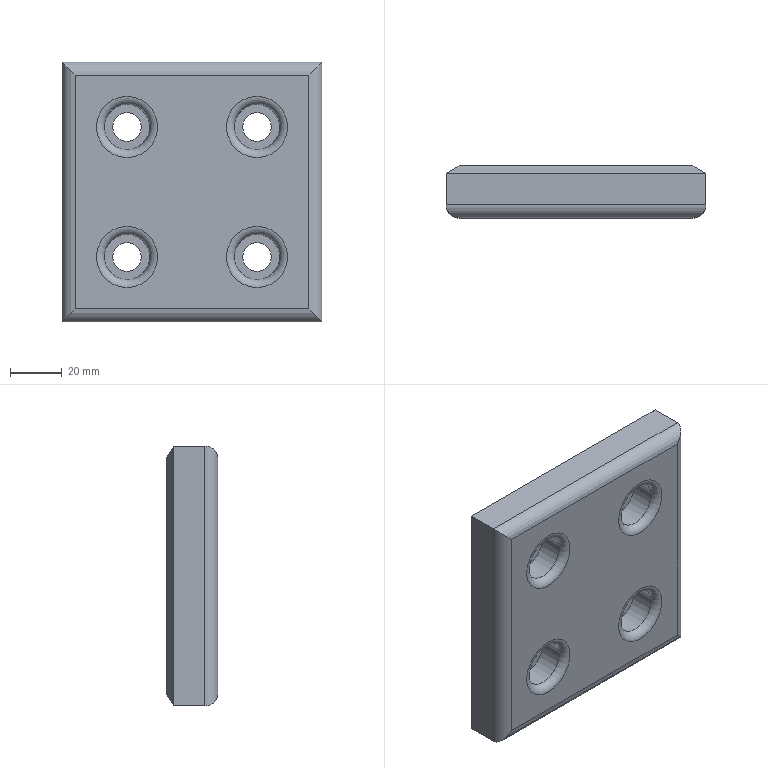Part | NX | features solid 2 | 1 solid | 30 faces | box 100 x 20 x 100 mm | volume 179958 mm3 | plane 14 | cylinder 12 | torus 4 | commonest cylinder face diameters 10 x4 11 x4 17.5 x4
STEP:
#1=CARTESIAN_POINT('',(395.,-583.,40.));
#2=VERTEX_POINT('',#1);
#3=CARTESIAN_POINT('',(395.,-595.,40.));
#4=VERTEX_POINT('',#3);
#5=CARTESIAN_POINT('',(395.,-580.,40.));
#6=DIRECTION('',(0.,-1.,0.));
#7=VECTOR('',#6,1000.);
#8=LINE('',#5,#7);
#9=EDGE_CURVE('',#2,#4,#8,.T.);
#10=ORIENTED_EDGE('',*,*,#9,.T.);
#11=CARTESIAN_POINT('',(395.,-595.,-60.));
#12=VERTEX_POINT('',#11);
#13=CARTESIAN_POINT('',(395.,-595.,90.));
#14=DIRECTION('',(0.,0.,-1.));
#15=VECTOR('',#14,1000.);
#16=LINE('',#13,#15);
#17=EDGE_CURVE('',#12,#4,#16,.F.);
#18=ORIENTED_EDGE('',*,*,#17,.F.);
#19=CARTESIAN_POINT('',(395.,-583.,-60.));
#20=VERTEX_POINT('',#19);
#21=CARTESIAN_POINT('',(395.,-580.,-60.));
#22=DIRECTION('',(0.,-1.,0.));
#23=VECTOR('',#22,1000.);
#24=LINE('',#21,#23);
#25=EDGE_CURVE('',#20,#12,#24,.T.);
#26=ORIENTED_EDGE('',*,*,#25,.F.);
#27=CARTESIAN_POINT('',(395.,-583.,-60.));
#28=DIRECTION('',(0.,0.,-1.));
#29=VECTOR('',#28,1000.);
#30=LINE('',#27,#29);
#31=EDGE_CURVE('',#2,#20,#30,.T.);
#32=ORIENTED_EDGE('',*,*,#31,.F.);
#33=EDGE_LOOP('',(#10,#18,#26,#32));
#34=FACE_BOUND('',#33,.T.);
#35=CARTESIAN_POINT('',(395.,-580.,90.));
#36=DIRECTION('',(1.,0.,0.));
#37=DIRECTION('',(0.,0.,1.));
#38=AXIS2_PLACEMENT_3D('',#35,#36,#37);
#39=PLANE('',#38);
#40=ADVANCED_FACE('',(#34),#39,.T.);
#41=CARTESIAN_POINT('',(295.,-583.,40.));
#42=VERTEX_POINT('',#41);
#43=CARTESIAN_POINT('',(295.,-595.,40.));
#44=VERTEX_POINT('',#43);
#45=CARTESIAN_POINT('',(295.,-580.,40.));
#46=DIRECTION('',(0.,-1.,0.));
#47=VECTOR('',#46,1000.);
#48=LINE('',#45,#47);
#49=EDGE_CURVE('',#42,#44,#48,.T.);
#50=ORIENTED_EDGE('',*,*,#49,.T.);
#51=CARTESIAN_POINT('',(295.,-595.,40.));
#52=DIRECTION('',(-1.,0.,0.));
#53=VECTOR('',#52,1000.);
#54=LINE('',#51,#53);
#55=EDGE_CURVE('',#4,#44,#54,.T.);
#56=ORIENTED_EDGE('',*,*,#55,.F.);
#57=ORIENTED_EDGE('',*,*,#9,.F.);
#58=CARTESIAN_POINT('',(395.,-583.,40.));
#59=DIRECTION('',(1.,0.,0.));
#60=VECTOR('',#59,1000.);
#61=LINE('',#58,#60);
#62=EDGE_CURVE('',#42,#2,#61,.T.);
#63=ORIENTED_EDGE('',*,*,#62,.F.);
#64=EDGE_LOOP('',(#50,#56,#57,#63));
#65=FACE_BOUND('',#64,.T.);
#66=CARTESIAN_POINT('',(395.,-580.,40.));
#67=DIRECTION('',(0.,0.,-1.));
#68=DIRECTION('',(1.,0.,0.));
#69=AXIS2_PLACEMENT_3D('',#66,#67,#68);
#70=PLANE('',#69);
#71=ADVANCED_FACE('',(#65),#70,.F.);
#72=CARTESIAN_POINT('',(295.,-583.,-60.));
#73=VERTEX_POINT('',#72);
#74=CARTESIAN_POINT('',(295.,-595.,-60.));
#75=VERTEX_POINT('',#74);
#76=CARTESIAN_POINT('',(295.,-580.,-60.));
#77=DIRECTION('',(0.,-1.,0.));
#78=VECTOR('',#77,1000.);
#79=LINE('',#76,#78);
#80=EDGE_CURVE('',#73,#75,#79,.T.);
#81=ORIENTED_EDGE('',*,*,#80,.T.);
#82=CARTESIAN_POINT('',(295.,-595.,-60.));
#83=DIRECTION('',(0.,0.,-1.));
#84=VECTOR('',#83,1000.);
#85=LINE('',#82,#84);
#86=EDGE_CURVE('',#44,#75,#85,.T.);
#87=ORIENTED_EDGE('',*,*,#86,.F.);
#88=ORIENTED_EDGE('',*,*,#49,.F.);
#89=CARTESIAN_POINT('',(295.,-583.,90.));
#90=DIRECTION('',(0.,0.,1.));
#91=VECTOR('',#90,1000.);
#92=LINE('',#89,#91);
#93=EDGE_CURVE('',#73,#42,#92,.T.);
#94=ORIENTED_EDGE('',*,*,#93,.F.);
#95=EDGE_LOOP('',(#81,#87,#88,#94));
#96=FACE_BOUND('',#95,.T.);
#97=CARTESIAN_POINT('',(295.,-580.,90.));
#98=DIRECTION('',(1.,0.,0.));
#99=DIRECTION('',(0.,0.,1.));
#100=AXIS2_PLACEMENT_3D('',#97,#98,#99);
#101=PLANE('',#100);
#102=ADVANCED_FACE('',(#96),#101,.F.);
#103=ORIENTED_EDGE('',*,*,#25,.T.);
#104=CARTESIAN_POINT('',(395.,-595.,-60.));
#105=DIRECTION('',(-1.,0.,0.));
#106=VECTOR('',#105,1000.);
#107=LINE('',#104,#106);
#108=EDGE_CURVE('',#75,#12,#107,.F.);
#109=ORIENTED_EDGE('',*,*,#108,.F.);
#110=ORIENTED_EDGE('',*,*,#80,.F.);
#111=CARTESIAN_POINT('',(295.,-583.,-60.));
#112=DIRECTION('',(-1.,0.,0.));
#113=VECTOR('',#112,1000.);
#114=LINE('',#111,#113);
#115=EDGE_CURVE('',#20,#73,#114,.T.);
#116=ORIENTED_EDGE('',*,*,#115,.F.);
#117=EDGE_LOOP('',(#103,#109,#110,#116));
#118=FACE_BOUND('',#117,.T.);
#119=CARTESIAN_POINT('',(395.,-580.,-60.));
#120=DIRECTION('',(0.,0.,-1.));
#121=DIRECTION('',(1.,0.,0.));
#122=AXIS2_PLACEMENT_3D('',#119,#120,#121);
#123=PLANE('',#122);
#124=ADVANCED_FACE('',(#118),#123,.T.);
#125=CARTESIAN_POINT('',(390.,-580.,35.));
#126=VERTEX_POINT('',#125);
#127=CARTESIAN_POINT('',(300.,-580.,35.));
#128=VERTEX_POINT('',#127);
#129=CARTESIAN_POINT('',(395.,-580.,35.));
#130=DIRECTION('',(-1.,0.,0.));
#131=VECTOR('',#130,1000.);
#132=LINE('',#129,#131);
#133=EDGE_CURVE('',#126,#128,#132,.T.);
#134=ORIENTED_EDGE('',*,*,#133,.F.);
#135=CARTESIAN_POINT('',(390.,-580.,-55.));
#136=VERTEX_POINT('',#135);
#137=CARTESIAN_POINT('',(390.,-580.,40.));
#138=DIRECTION('',(0.,0.,1.));
#139=VECTOR('',#138,1000.);
#140=LINE('',#137,#139);
#141=EDGE_CURVE('',#136,#126,#140,.T.);
#142=ORIENTED_EDGE('',*,*,#141,.F.);
#143=CARTESIAN_POINT('',(300.,-580.,-55.));
#144=VERTEX_POINT('',#143);
#145=CARTESIAN_POINT('',(395.,-580.,-55.));
#146=DIRECTION('',(1.,0.,0.));
#147=VECTOR('',#146,1000.);
#148=LINE('',#145,#147);
#149=EDGE_CURVE('',#144,#136,#148,.T.);
#150=ORIENTED_EDGE('',*,*,#149,.F.);
#151=CARTESIAN_POINT('',(300.,-580.,90.));
#152=DIRECTION('',(0.,0.,-1.));
#153=VECTOR('',#152,1000.);
#154=LINE('',#151,#153);
#155=EDGE_CURVE('',#128,#144,#154,.T.);
#156=ORIENTED_EDGE('',*,*,#155,.F.);
#157=EDGE_LOOP('',(#134,#142,#150,#156));
#158=FACE_BOUND('',#157,.T.);
#159=CARTESIAN_POINT('',(320.,-580.,-40.5));
#160=VERTEX_POINT('',#159);
#161=CARTESIAN_POINT('',(320.,-580.,-35.));
#162=DIRECTION('',(0.,1.,0.));
#163=DIRECTION('',(0.,0.,-1.));
#164=AXIS2_PLACEMENT_3D('',#161,#162,#163);
#165=CIRCLE('',#164,5.5);
#166=EDGE_CURVE('',#160,#160,#165,.T.);
#167=ORIENTED_EDGE('',*,*,#166,.F.);
#168=EDGE_LOOP('',(#167));
#169=FACE_BOUND('',#168,.T.);
#170=CARTESIAN_POINT('',(370.,-580.,-40.5));
#171=VERTEX_POINT('',#170);
#172=CARTESIAN_POINT('',(370.,-580.,-35.));
#173=DIRECTION('',(0.,1.,0.));
#174=DIRECTION('',(0.,0.,-1.));
#175=AXIS2_PLACEMENT_3D('',#172,#173,#174);
#176=CIRCLE('',#175,5.5);
#177=EDGE_CURVE('',#171,#171,#176,.T.);
#178=ORIENTED_EDGE('',*,*,#177,.F.);
#179=EDGE_LOOP('',(#178));
#180=FACE_BOUND('',#179,.T.);
#181=CARTESIAN_POINT('',(320.,-580.,9.5));
#182=VERTEX_POINT('',#181);
#183=CARTESIAN_POINT('',(320.,-580.,15.));
#184=DIRECTION('',(0.,1.,0.));
#185=DIRECTION('',(0.,0.,-1.));
#186=AXIS2_PLACEMENT_3D('',#183,#184,#185);
#187=CIRCLE('',#186,5.5);
#188=EDGE_CURVE('',#182,#182,#187,.T.);
#189=ORIENTED_EDGE('',*,*,#188,.F.);
#190=EDGE_LOOP('',(#189));
#191=FACE_BOUND('',#190,.T.);
#192=CARTESIAN_POINT('',(370.,-580.,9.5));
#193=VERTEX_POINT('',#192);
#194=CARTESIAN_POINT('',(370.,-580.,15.));
#195=DIRECTION('',(0.,1.,0.));
#196=DIRECTION('',(0.,0.,-1.));
#197=AXIS2_PLACEMENT_3D('',#194,#195,#196);
#198=CIRCLE('',#197,5.5);
#199=EDGE_CURVE('',#193,#193,#198,.T.);
#200=ORIENTED_EDGE('',*,*,#199,.F.);
#201=EDGE_LOOP('',(#200));
#202=FACE_BOUND('',#201,.T.);
#203=CARTESIAN_POINT('',(395.,-580.,90.));
#204=DIRECTION('',(0.,-1.,0.));
#205=DIRECTION('',(-1.,0.,0.));
#206=AXIS2_PLACEMENT_3D('',#203,#204,#205);
#207=PLANE('',#206);
#208=ADVANCED_FACE('',(#158,#169,#180,#191,#202),#207,.F.);
#209=CARTESIAN_POINT('',(370.,-600.,-46.75));
#210=VERTEX_POINT('',#209);
#211=CARTESIAN_POINT('',(370.,-600.,-35.));
#212=DIRECTION('',(0.,1.,0.));
#213=DIRECTION('',(0.,0.,-1.));
#214=AXIS2_PLACEMENT_3D('',#211,#212,#213);
#215=CIRCLE('',#214,11.75);
#216=EDGE_CURVE('',#210,#210,#215,.F.);
#217=ORIENTED_EDGE('',*,*,#216,.F.);
#218=EDGE_LOOP('',(#217));
#219=FACE_BOUND('',#218,.T.);
#220=CARTESIAN_POINT('',(320.,-600.,-46.75));
#221=VERTEX_POINT('',#220);
#222=CARTESIAN_POINT('',(320.,-600.,-35.));
#223=DIRECTION('',(0.,1.,0.));
#224=DIRECTION('',(0.,0.,-1.));
#225=AXIS2_PLACEMENT_3D('',#222,#223,#224);
#226=CIRCLE('',#225,11.75);
#227=EDGE_CURVE('',#221,#221,#226,.F.);
#228=ORIENTED_EDGE('',*,*,#227,.F.);
#229=EDGE_LOOP('',(#228));
#230=FACE_BOUND('',#229,.T.);
#231=CARTESIAN_POINT('',(320.,-600.,3.25));
#232=VERTEX_POINT('',#231);
#233=CARTESIAN_POINT('',(320.,-600.,15.));
#234=DIRECTION('',(0.,1.,0.));
#235=DIRECTION('',(0.,0.,-1.));
#236=AXIS2_PLACEMENT_3D('',#233,#234,#235);
#237=CIRCLE('',#236,11.75);
#238=EDGE_CURVE('',#232,#232,#237,.F.);
#239=ORIENTED_EDGE('',*,*,#238,.F.);
#240=EDGE_LOOP('',(#239));
#241=FACE_BOUND('',#240,.T.);
#242=CARTESIAN_POINT('',(370.,-600.,3.25));
#243=VERTEX_POINT('',#242);
#244=CARTESIAN_POINT('',(370.,-600.,15.));
#245=DIRECTION('',(0.,1.,0.));
#246=DIRECTION('',(0.,0.,-1.));
#247=AXIS2_PLACEMENT_3D('',#244,#245,#246);
#248=CIRCLE('',#247,11.75);
#249=EDGE_CURVE('',#243,#243,#248,.F.);
#250=ORIENTED_EDGE('',*,*,#249,.F.);
#251=EDGE_LOOP('',(#250));
#252=FACE_BOUND('',#251,.T.);
#253=CARTESIAN_POINT('',(390.,-600.,35.));
#254=VERTEX_POINT('',#253);
#255=CARTESIAN_POINT('',(390.,-600.,-55.));
#256=VERTEX_POINT('',#255);
#257=CARTESIAN_POINT('',(390.,-600.,90.));
#258=DIRECTION('',(0.,0.,-1.));
#259=VECTOR('',#258,1000.);
#260=LINE('',#257,#259);
#261=EDGE_CURVE('',#254,#256,#260,.T.);
#262=ORIENTED_EDGE('',*,*,#261,.F.);
#263=CARTESIAN_POINT('',(300.,-600.,35.));
#264=VERTEX_POINT('',#263);
#265=CARTESIAN_POINT('',(395.,-600.,35.));
#266=DIRECTION('',(-1.,0.,0.));
#267=VECTOR('',#266,1000.);
#268=LINE('',#265,#267);
#269=EDGE_CURVE('',#264,#254,#268,.F.);
#270=ORIENTED_EDGE('',*,*,#269,.F.);
#271=CARTESIAN_POINT('',(300.,-600.,-55.));
#272=VERTEX_POINT('',#271);
#273=CARTESIAN_POINT('',(300.,-600.,40.));
#274=DIRECTION('',(0.,0.,-1.));
#275=VECTOR('',#274,1000.);
#276=LINE('',#273,#275);
#277=EDGE_CURVE('',#272,#264,#276,.F.);
#278=ORIENTED_EDGE('',*,*,#277,.F.);
#279=CARTESIAN_POINT('',(395.,-600.,-55.));
#280=DIRECTION('',(-1.,0.,0.));
#281=VECTOR('',#280,1000.);
#282=LINE('',#279,#281);
#283=EDGE_CURVE('',#256,#272,#282,.T.);
#284=ORIENTED_EDGE('',*,*,#283,.F.);
#285=EDGE_LOOP('',(#262,#270,#278,#284));
#286=FACE_BOUND('',#285,.T.);
#287=CARTESIAN_POINT('',(395.,-600.,90.));
#288=DIRECTION('',(0.,-1.,0.));
#289=DIRECTION('',(-1.,0.,0.));
#290=AXIS2_PLACEMENT_3D('',#287,#288,#289);
#291=PLANE('',#290);
#292=ADVANCED_FACE('',(#219,#230,#241,#252,#286),#291,.T.);
#293=CARTESIAN_POINT('',(370.,-588.,20.5));
#294=VERTEX_POINT('',#293);
#295=CARTESIAN_POINT('',(370.,-588.,15.));
#296=DIRECTION('',(0.,-1.,0.));
#297=DIRECTION('',(0.,0.,1.));
#298=AXIS2_PLACEMENT_3D('',#295,#296,#297);
#299=CIRCLE('',#298,5.5);
#300=EDGE_CURVE('',#294,#294,#299,.T.);
#301=ORIENTED_EDGE('',*,*,#300,.T.);
#302=EDGE_LOOP('',(#301));
#303=FACE_BOUND('',#302,.T.);
#304=ORIENTED_EDGE('',*,*,#199,.T.);
#305=EDGE_LOOP('',(#304));
#306=FACE_BOUND('',#305,.T.);
#307=CARTESIAN_POINT('',(370.,-550.,15.));
#308=DIRECTION('',(0.,1.,0.));
#309=DIRECTION('',(0.,0.,1.));
#310=AXIS2_PLACEMENT_3D('',#307,#308,#309);
#311=CYLINDRICAL_SURFACE('',#310,5.5);
#312=ADVANCED_FACE('',(#303,#306),#311,.F.);
#313=ORIENTED_EDGE('',*,*,#300,.F.);
#314=EDGE_LOOP('',(#313));
#315=FACE_BOUND('',#314,.T.);
#316=CARTESIAN_POINT('',(370.,-588.,23.75));
#317=VERTEX_POINT('',#316);
#318=CARTESIAN_POINT('',(370.,-588.,15.));
#319=DIRECTION('',(0.,-1.,0.));
#320=DIRECTION('',(0.,0.,1.));
#321=AXIS2_PLACEMENT_3D('',#318,#319,#320);
#322=CIRCLE('',#321,8.75);
#323=EDGE_CURVE('',#317,#317,#322,.T.);
#324=ORIENTED_EDGE('',*,*,#323,.T.);
#325=EDGE_LOOP('',(#324));
#326=FACE_BOUND('',#325,.T.);
#327=CARTESIAN_POINT('',(370.,-588.,15.));
#328=DIRECTION('',(0.,1.,0.));
#329=DIRECTION('',(0.,0.,1.));
#330=AXIS2_PLACEMENT_3D('',#327,#328,#329);
#331=PLANE('',#330);
#332=ADVANCED_FACE('',(#315,#326),#331,.F.);
#333=CARTESIAN_POINT('',(370.,-597.,6.25));
#334=VERTEX_POINT('',#333);
#335=CARTESIAN_POINT('',(370.,-597.,15.));
#336=DIRECTION('',(0.,1.,0.));
#337=DIRECTION('',(0.,0.,-1.));
#338=AXIS2_PLACEMENT_3D('',#335,#336,#337);
#339=CIRCLE('',#338,8.75);
#340=EDGE_CURVE('',#334,#334,#339,.T.);
#341=ORIENTED_EDGE('',*,*,#340,.F.);
#342=EDGE_LOOP('',(#341));
#343=FACE_BOUND('',#342,.T.);
#344=ORIENTED_EDGE('',*,*,#323,.F.);
#345=EDGE_LOOP('',(#344));
#346=FACE_BOUND('',#345,.T.);
#347=CARTESIAN_POINT('',(370.,-600.,15.));
#348=DIRECTION('',(0.,1.,0.));
#349=DIRECTION('',(0.,0.,1.));
#350=AXIS2_PLACEMENT_3D('',#347,#348,#349);
#351=CYLINDRICAL_SURFACE('',#350,8.75);
#352=ADVANCED_FACE('',(#343,#346),#351,.F.);
#353=CARTESIAN_POINT('',(320.,-588.,20.5));
#354=VERTEX_POINT('',#353);
#355=CARTESIAN_POINT('',(320.,-588.,15.));
#356=DIRECTION('',(0.,-1.,0.));
#357=DIRECTION('',(0.,0.,1.));
#358=AXIS2_PLACEMENT_3D('',#355,#356,#357);
#359=CIRCLE('',#358,5.5);
#360=EDGE_CURVE('',#354,#354,#359,.T.);
#361=ORIENTED_EDGE('',*,*,#360,.T.);
#362=EDGE_LOOP('',(#361));
#363=FACE_BOUND('',#362,.T.);
#364=ORIENTED_EDGE('',*,*,#188,.T.);
#365=EDGE_LOOP('',(#364));
#366=FACE_BOUND('',#365,.T.);
#367=CARTESIAN_POINT('',(320.,-550.,15.));
#368=DIRECTION('',(0.,1.,0.));
#369=DIRECTION('',(0.,0.,1.));
#370=AXIS2_PLACEMENT_3D('',#367,#368,#369);
#371=CYLINDRICAL_SURFACE('',#370,5.5);
#372=ADVANCED_FACE('',(#363,#366),#371,.F.);
#373=ORIENTED_EDGE('',*,*,#360,.F.);
#374=EDGE_LOOP('',(#373));
#375=FACE_BOUND('',#374,.T.);
#376=CARTESIAN_POINT('',(320.,-588.,23.75));
#377=VERTEX_POINT('',#376);
#378=CARTESIAN_POINT('',(320.,-588.,15.));
#379=DIRECTION('',(0.,-1.,0.));
#380=DIRECTION('',(0.,0.,1.));
#381=AXIS2_PLACEMENT_3D('',#378,#379,#380);
#382=CIRCLE('',#381,8.75);
#383=EDGE_CURVE('',#377,#377,#382,.T.);
#384=ORIENTED_EDGE('',*,*,#383,.T.);
#385=EDGE_LOOP('',(#384));
#386=FACE_BOUND('',#385,.T.);
#387=CARTESIAN_POINT('',(320.,-588.,15.));
#388=DIRECTION('',(0.,1.,0.));
#389=DIRECTION('',(0.,0.,1.));
#390=AXIS2_PLACEMENT_3D('',#387,#388,#389);
#391=PLANE('',#390);
#392=ADVANCED_FACE('',(#375,#386),#391,.F.);
#393=CARTESIAN_POINT('',(320.,-597.,6.25));
#394=VERTEX_POINT('',#393);
#395=CARTESIAN_POINT('',(320.,-597.,15.));
#396=DIRECTION('',(0.,1.,0.));
#397=DIRECTION('',(0.,0.,-1.));
#398=AXIS2_PLACEMENT_3D('',#395,#396,#397);
#399=CIRCLE('',#398,8.75);
#400=EDGE_CURVE('',#394,#394,#399,.T.);
#401=ORIENTED_EDGE('',*,*,#400,.F.);
#402=EDGE_LOOP('',(#401));
#403=FACE_BOUND('',#402,.T.);
#404=ORIENTED_EDGE('',*,*,#383,.F.);
#405=EDGE_LOOP('',(#404));
#406=FACE_BOUND('',#405,.T.);
#407=CARTESIAN_POINT('',(320.,-600.,15.));
#408=DIRECTION('',(0.,1.,0.));
#409=DIRECTION('',(0.,0.,1.));
#410=AXIS2_PLACEMENT_3D('',#407,#408,#409);
#411=CYLINDRICAL_SURFACE('',#410,8.75);
#412=ADVANCED_FACE('',(#403,#406),#411,.F.);
#413=CARTESIAN_POINT('',(370.,-588.,-29.5));
#414=VERTEX_POINT('',#413);
#415=CARTESIAN_POINT('',(370.,-588.,-35.));
#416=DIRECTION('',(0.,-1.,0.));
#417=DIRECTION('',(0.,0.,1.));
#418=AXIS2_PLACEMENT_3D('',#415,#416,#417);
#419=CIRCLE('',#418,5.5);
#420=EDGE_CURVE('',#414,#414,#419,.T.);
#421=ORIENTED_EDGE('',*,*,#420,.T.);
#422=EDGE_LOOP('',(#421));
#423=FACE_BOUND('',#422,.T.);
#424=ORIENTED_EDGE('',*,*,#177,.T.);
#425=EDGE_LOOP('',(#424));
#426=FACE_BOUND('',#425,.T.);
#427=CARTESIAN_POINT('',(370.,-550.,-35.));
#428=DIRECTION('',(0.,1.,0.));
#429=DIRECTION('',(0.,0.,1.));
#430=AXIS2_PLACEMENT_3D('',#427,#428,#429);
#431=CYLINDRICAL_SURFACE('',#430,5.5);
#432=ADVANCED_FACE('',(#423,#426),#431,.F.);
#433=ORIENTED_EDGE('',*,*,#420,.F.);
#434=EDGE_LOOP('',(#433));
#435=FACE_BOUND('',#434,.T.);
#436=CARTESIAN_POINT('',(370.,-588.,-26.25));
#437=VERTEX_POINT('',#436);
#438=CARTESIAN_POINT('',(370.,-588.,-35.));
#439=DIRECTION('',(0.,-1.,0.));
#440=DIRECTION('',(0.,0.,1.));
#441=AXIS2_PLACEMENT_3D('',#438,#439,#440);
#442=CIRCLE('',#441,8.75);
#443=EDGE_CURVE('',#437,#437,#442,.T.);
#444=ORIENTED_EDGE('',*,*,#443,.T.);
#445=EDGE_LOOP('',(#444));
#446=FACE_BOUND('',#445,.T.);
#447=CARTESIAN_POINT('',(370.,-588.,-35.));
#448=DIRECTION('',(0.,1.,0.));
#449=DIRECTION('',(0.,0.,1.));
#450=AXIS2_PLACEMENT_3D('',#447,#448,#449);
#451=PLANE('',#450);
#452=ADVANCED_FACE('',(#435,#446),#451,.F.);
#453=CARTESIAN_POINT('',(370.,-597.,-43.75));
#454=VERTEX_POINT('',#453);
#455=CARTESIAN_POINT('',(370.,-597.,-35.));
#456=DIRECTION('',(0.,1.,0.));
#457=DIRECTION('',(0.,0.,-1.));
#458=AXIS2_PLACEMENT_3D('',#455,#456,#457);
#459=CIRCLE('',#458,8.75);
#460=EDGE_CURVE('',#454,#454,#459,.T.);
#461=ORIENTED_EDGE('',*,*,#460,.F.);
#462=EDGE_LOOP('',(#461));
#463=FACE_BOUND('',#462,.T.);
#464=ORIENTED_EDGE('',*,*,#443,.F.);
#465=EDGE_LOOP('',(#464));
#466=FACE_BOUND('',#465,.T.);
#467=CARTESIAN_POINT('',(370.,-600.,-35.));
#468=DIRECTION('',(0.,1.,0.));
#469=DIRECTION('',(0.,0.,1.));
#470=AXIS2_PLACEMENT_3D('',#467,#468,#469);
#471=CYLINDRICAL_SURFACE('',#470,8.75);
#472=ADVANCED_FACE('',(#463,#466),#471,.F.);
#473=CARTESIAN_POINT('',(320.,-588.,-29.5));
#474=VERTEX_POINT('',#473);
#475=CARTESIAN_POINT('',(320.,-588.,-35.));
#476=DIRECTION('',(0.,-1.,0.));
#477=DIRECTION('',(0.,0.,1.));
#478=AXIS2_PLACEMENT_3D('',#475,#476,#477);
#479=CIRCLE('',#478,5.5);
#480=EDGE_CURVE('',#474,#474,#479,.T.);
#481=ORIENTED_EDGE('',*,*,#480,.T.);
#482=EDGE_LOOP('',(#481));
#483=FACE_BOUND('',#482,.T.);
#484=ORIENTED_EDGE('',*,*,#166,.T.);
#485=EDGE_LOOP('',(#484));
#486=FACE_BOUND('',#485,.T.);
#487=CARTESIAN_POINT('',(320.,-550.,-35.));
#488=DIRECTION('',(0.,1.,0.));
#489=DIRECTION('',(0.,0.,1.));
#490=AXIS2_PLACEMENT_3D('',#487,#488,#489);
#491=CYLINDRICAL_SURFACE('',#490,5.5);
#492=ADVANCED_FACE('',(#483,#486),#491,.F.);
#493=ORIENTED_EDGE('',*,*,#480,.F.);
#494=EDGE_LOOP('',(#493));
#495=FACE_BOUND('',#494,.T.);
#496=CARTESIAN_POINT('',(320.,-588.,-26.25));
#497=VERTEX_POINT('',#496);
#498=CARTESIAN_POINT('',(320.,-588.,-35.));
#499=DIRECTION('',(0.,-1.,0.));
#500=DIRECTION('',(0.,0.,1.));
#501=AXIS2_PLACEMENT_3D('',#498,#499,#500);
#502=CIRCLE('',#501,8.75);
#503=EDGE_CURVE('',#497,#497,#502,.T.);
#504=ORIENTED_EDGE('',*,*,#503,.T.);
#505=EDGE_LOOP('',(#504));
#506=FACE_BOUND('',#505,.T.);
#507=CARTESIAN_POINT('',(320.,-588.,-35.));
#508=DIRECTION('',(0.,1.,0.));
#509=DIRECTION('',(0.,0.,1.));
#510=AXIS2_PLACEMENT_3D('',#507,#508,#509);
#511=PLANE('',#510);
#512=ADVANCED_FACE('',(#495,#506),#511,.F.);
#513=CARTESIAN_POINT('',(320.,-597.,-43.75));
#514=VERTEX_POINT('',#513);
#515=CARTESIAN_POINT('',(320.,-597.,-35.));
#516=DIRECTION('',(0.,1.,0.));
#517=DIRECTION('',(0.,0.,-1.));
#518=AXIS2_PLACEMENT_3D('',#515,#516,#517);
#519=CIRCLE('',#518,8.75);
#520=EDGE_CURVE('',#514,#514,#519,.T.);
#521=ORIENTED_EDGE('',*,*,#520,.F.);
#522=EDGE_LOOP('',(#521));
#523=FACE_BOUND('',#522,.T.);
#524=ORIENTED_EDGE('',*,*,#503,.F.);
#525=EDGE_LOOP('',(#524));
#526=FACE_BOUND('',#525,.T.);
#527=CARTESIAN_POINT('',(320.,-600.,-35.));
#528=DIRECTION('',(0.,1.,0.));
#529=DIRECTION('',(0.,0.,1.));
#530=AXIS2_PLACEMENT_3D('',#527,#528,#529);
#531=CYLINDRICAL_SURFACE('',#530,8.75);
#532=ADVANCED_FACE('',(#523,#526),#531,.F.);
#533=CARTESIAN_POINT('',(300.,-595.,35.));
#534=DIRECTION('',(-0.7071,0.,-0.7071));
#535=DIRECTION('',(0.7071,0.,-0.7071));
#536=AXIS2_PLACEMENT_3D('',#533,#534,#535);
#537=ELLIPSE('',#536,7.071,5.);
#538=EDGE_CURVE('',#44,#264,#537,.F.);
#539=ORIENTED_EDGE('',*,*,#538,.T.);
#540=ORIENTED_EDGE('',*,*,#269,.T.);
#541=CARTESIAN_POINT('',(390.,-595.,35.));
#542=DIRECTION('',(-0.7071,0.,0.7071));
#543=DIRECTION('',(-0.7071,0.,-0.7071));
#544=AXIS2_PLACEMENT_3D('',#541,#542,#543);
#545=ELLIPSE('',#544,7.071,5.);
#546=EDGE_CURVE('',#254,#4,#545,.T.);
#547=ORIENTED_EDGE('',*,*,#546,.T.);
#548=ORIENTED_EDGE('',*,*,#55,.T.);
#549=EDGE_LOOP('',(#539,#540,#547,#548));
#550=FACE_BOUND('',#549,.T.);
#551=CARTESIAN_POINT('',(395.,-595.,35.));
#552=DIRECTION('',(1.,0.,0.));
#553=DIRECTION('',(0.,0.,1.));
#554=AXIS2_PLACEMENT_3D('',#551,#552,#553);
#555=CYLINDRICAL_SURFACE('',#554,5.);
#556=ADVANCED_FACE('',(#550),#555,.T.);
#557=ORIENTED_EDGE('',*,*,#546,.F.);
#558=ORIENTED_EDGE('',*,*,#261,.T.);
#559=CARTESIAN_POINT('',(390.,-595.,-55.));
#560=DIRECTION('',(0.7071,0.,0.7071));
#561=DIRECTION('',(0.7071,0.,-0.7071));
#562=AXIS2_PLACEMENT_3D('',#559,#560,#561);
#563=ELLIPSE('',#562,7.071,5.);
#564=EDGE_CURVE('',#256,#12,#563,.T.);
#565=ORIENTED_EDGE('',*,*,#564,.T.);
#566=ORIENTED_EDGE('',*,*,#17,.T.);
#567=EDGE_LOOP('',(#557,#558,#565,#566));
#568=FACE_BOUND('',#567,.T.);
#569=CARTESIAN_POINT('',(390.,-595.,90.));
#570=DIRECTION('',(0.,0.,-1.));
#571=DIRECTION('',(1.,0.,0.));
#572=AXIS2_PLACEMENT_3D('',#569,#570,#571);
#573=CYLINDRICAL_SURFACE('',#572,5.);
#574=ADVANCED_FACE('',(#568),#573,.T.);
#575=ORIENTED_EDGE('',*,*,#538,.F.);
#576=ORIENTED_EDGE('',*,*,#86,.T.);
#577=CARTESIAN_POINT('',(300.,-595.,-55.));
#578=DIRECTION('',(0.7071,0.,-0.7071));
#579=DIRECTION('',(0.7071,0.,0.7071));
#580=AXIS2_PLACEMENT_3D('',#577,#578,#579);
#581=ELLIPSE('',#580,7.071,5.);
#582=EDGE_CURVE('',#75,#272,#581,.F.);
#583=ORIENTED_EDGE('',*,*,#582,.T.);
#584=ORIENTED_EDGE('',*,*,#277,.T.);
#585=EDGE_LOOP('',(#575,#576,#583,#584));
#586=FACE_BOUND('',#585,.T.);
#587=CARTESIAN_POINT('',(300.,-595.,90.));
#588=DIRECTION('',(0.,0.,1.));
#589=DIRECTION('',(-1.,0.,0.));
#590=AXIS2_PLACEMENT_3D('',#587,#588,#589);
#591=CYLINDRICAL_SURFACE('',#590,5.);
#592=ADVANCED_FACE('',(#586),#591,.T.);
#593=ORIENTED_EDGE('',*,*,#564,.F.);
#594=ORIENTED_EDGE('',*,*,#283,.T.);
#595=ORIENTED_EDGE('',*,*,#582,.F.);
#596=ORIENTED_EDGE('',*,*,#108,.T.);
#597=EDGE_LOOP('',(#593,#594,#595,#596));
#598=FACE_BOUND('',#597,.T.);
#599=CARTESIAN_POINT('',(395.,-595.,-55.));
#600=DIRECTION('',(-1.,0.,0.));
#601=DIRECTION('',(0.,0.,-1.));
#602=AXIS2_PLACEMENT_3D('',#599,#600,#601);
#603=CYLINDRICAL_SURFACE('',#602,5.);
#604=ADVANCED_FACE('',(#598),#603,.T.);
#605=ORIENTED_EDGE('',*,*,#460,.T.);
#606=EDGE_LOOP('',(#605));
#607=FACE_BOUND('',#606,.T.);
#608=ORIENTED_EDGE('',*,*,#216,.T.);
#609=EDGE_LOOP('',(#608));
#610=FACE_BOUND('',#609,.T.);
#611=CARTESIAN_POINT('',(370.,-597.,-35.));
#612=DIRECTION('',(0.,-1.,0.));
#613=DIRECTION('',(0.,0.,-1.));
#614=AXIS2_PLACEMENT_3D('',#611,#612,#613);
#615=TOROIDAL_SURFACE('',#614,11.75,3.);
#616=ADVANCED_FACE('',(#607,#610),#615,.T.);
#617=ORIENTED_EDGE('',*,*,#520,.T.);
#618=EDGE_LOOP('',(#617));
#619=FACE_BOUND('',#618,.T.);
#620=ORIENTED_EDGE('',*,*,#227,.T.);
#621=EDGE_LOOP('',(#620));
#622=FACE_BOUND('',#621,.T.);
#623=CARTESIAN_POINT('',(320.,-597.,-35.));
#624=DIRECTION('',(0.,-1.,0.));
#625=DIRECTION('',(0.,0.,-1.));
#626=AXIS2_PLACEMENT_3D('',#623,#624,#625);
#627=TOROIDAL_SURFACE('',#626,11.75,3.);
#628=ADVANCED_FACE('',(#619,#622),#627,.T.);
#629=ORIENTED_EDGE('',*,*,#400,.T.);
#630=EDGE_LOOP('',(#629));
#631=FACE_BOUND('',#630,.T.);
#632=ORIENTED_EDGE('',*,*,#238,.T.);
#633=EDGE_LOOP('',(#632));
#634=FACE_BOUND('',#633,.T.);
#635=CARTESIAN_POINT('',(320.,-597.,15.));
#636=DIRECTION('',(0.,-1.,0.));
#637=DIRECTION('',(0.,0.,-1.));
#638=AXIS2_PLACEMENT_3D('',#635,#636,#637);
#639=TOROIDAL_SURFACE('',#638,11.75,3.);
#640=ADVANCED_FACE('',(#631,#634),#639,.T.);
#641=ORIENTED_EDGE('',*,*,#340,.T.);
#642=EDGE_LOOP('',(#641));
#643=FACE_BOUND('',#642,.T.);
#644=ORIENTED_EDGE('',*,*,#249,.T.);
#645=EDGE_LOOP('',(#644));
#646=FACE_BOUND('',#645,.T.);
#647=CARTESIAN_POINT('',(370.,-597.,15.));
#648=DIRECTION('',(0.,-1.,0.));
#649=DIRECTION('',(0.,0.,-1.));
#650=AXIS2_PLACEMENT_3D('',#647,#648,#649);
#651=TOROIDAL_SURFACE('',#650,11.75,3.);
#652=ADVANCED_FACE('',(#643,#646),#651,.T.);
#653=CARTESIAN_POINT('',(331.441,-544.864,3.559));
#654=DIRECTION('',(0.6509,-0.3906,-0.6509));
#655=VECTOR('',#654,1000.);
#656=LINE('',#653,#655);
#657=EDGE_CURVE('',#20,#136,#656,.F.);
#658=ORIENTED_EDGE('',*,*,#657,.T.);
#659=ORIENTED_EDGE('',*,*,#141,.T.);
#660=CARTESIAN_POINT('',(416.186,-595.712,61.186));
#661=DIRECTION('',(0.6509,-0.3906,0.6509));
#662=VECTOR('',#661,1000.);
#663=LINE('',#660,#662);
#664=EDGE_CURVE('',#126,#2,#663,.T.);
#665=ORIENTED_EDGE('',*,*,#664,.T.);
#666=ORIENTED_EDGE('',*,*,#31,.T.);
#667=EDGE_LOOP('',(#658,#659,#665,#666));
#668=FACE_BOUND('',#667,.T.);
#669=CARTESIAN_POINT('',(395.,-583.,90.));
#670=DIRECTION('',(0.5145,0.8575,0.));
#671=DIRECTION('',(0.8575,-0.5145,0.));
#672=AXIS2_PLACEMENT_3D('',#669,#670,#671);
#673=PLANE('',#672);
#674=ADVANCED_FACE('',(#668),#673,.T.);
#675=ORIENTED_EDGE('',*,*,#664,.F.);
#676=ORIENTED_EDGE('',*,*,#133,.T.);
#677=CARTESIAN_POINT('',(340.254,-555.847,-5.254));
#678=DIRECTION('',(0.6509,0.3906,-0.6509));
#679=VECTOR('',#678,1000.);
#680=LINE('',#677,#679);
#681=EDGE_CURVE('',#128,#42,#680,.F.);
#682=ORIENTED_EDGE('',*,*,#681,.T.);
#683=ORIENTED_EDGE('',*,*,#62,.T.);
#684=EDGE_LOOP('',(#675,#676,#682,#683));
#685=FACE_BOUND('',#684,.T.);
#686=CARTESIAN_POINT('',(395.,-580.,35.));
#687=DIRECTION('',(0.,-0.8575,-0.5145));
#688=DIRECTION('',(0.,0.5145,-0.8575));
#689=AXIS2_PLACEMENT_3D('',#686,#687,#688);
#690=PLANE('',#689);
#691=ADVANCED_FACE('',(#685),#690,.F.);
#692=ORIENTED_EDGE('',*,*,#657,.F.);
#693=ORIENTED_EDGE('',*,*,#115,.T.);
#694=CARTESIAN_POINT('',(337.373,-557.576,-17.627));
#695=DIRECTION('',(0.6509,0.3906,0.6509));
#696=VECTOR('',#695,1000.);
#697=LINE('',#694,#696);
#698=EDGE_CURVE('',#73,#144,#697,.T.);
#699=ORIENTED_EDGE('',*,*,#698,.T.);
#700=ORIENTED_EDGE('',*,*,#149,.T.);
#701=EDGE_LOOP('',(#692,#693,#699,#700));
#702=FACE_BOUND('',#701,.T.);
#703=CARTESIAN_POINT('',(395.,-583.,-60.));
#704=DIRECTION('',(0.,0.8575,-0.5145));
#705=DIRECTION('',(0.,0.5145,0.8575));
#706=AXIS2_PLACEMENT_3D('',#703,#704,#705);
#707=PLANE('',#706);
#708=ADVANCED_FACE('',(#702),#707,.T.);
#709=ORIENTED_EDGE('',*,*,#681,.F.);
#710=ORIENTED_EDGE('',*,*,#155,.T.);
#711=ORIENTED_EDGE('',*,*,#698,.F.);
#712=ORIENTED_EDGE('',*,*,#93,.T.);
#713=EDGE_LOOP('',(#709,#710,#711,#712));
#714=FACE_BOUND('',#713,.T.);
#715=CARTESIAN_POINT('',(300.,-580.,90.));
#716=DIRECTION('',(0.5145,-0.8575,0.));
#717=DIRECTION('',(-0.8575,-0.5145,0.));
#718=AXIS2_PLACEMENT_3D('',#715,#716,#717);
#719=PLANE('',#718);
#720=ADVANCED_FACE('',(#714),#719,.F.);
#721=CLOSED_SHELL('',(#40,#71,#102,#124,#208,#292,#312,#332,#352,#372,#392,#412,#432,#452,#472,#492,#512,#532,#556,#574,#592,#604,#616,#628,#640,#652,#674,#691,#708,#720));
#722=MANIFOLD_SOLID_BREP('',#721);
#723=(LENGTH_UNIT()NAMED_UNIT(*)SI_UNIT(.MILLI.,.METRE.));
#724=UNCERTAINTY_MEASURE_WITH_UNIT(LENGTH_MEASURE(0.00001),#723,'','');
#725=(NAMED_UNIT(*)PLANE_ANGLE_UNIT()SI_UNIT($,.RADIAN.));
#726=(NAMED_UNIT(*)SI_UNIT($,.STERADIAN.)SOLID_ANGLE_UNIT());
#727=(GEOMETRIC_REPRESENTATION_CONTEXT(3)GLOBAL_UNCERTAINTY_ASSIGNED_CONTEXT((#724))GLOBAL_UNIT_ASSIGNED_CONTEXT((#723,#725,#726))REPRESENTATION_CONTEXT('',''));
#728=ADVANCED_BREP_SHAPE_REPRESENTATION('',(#722),#727);